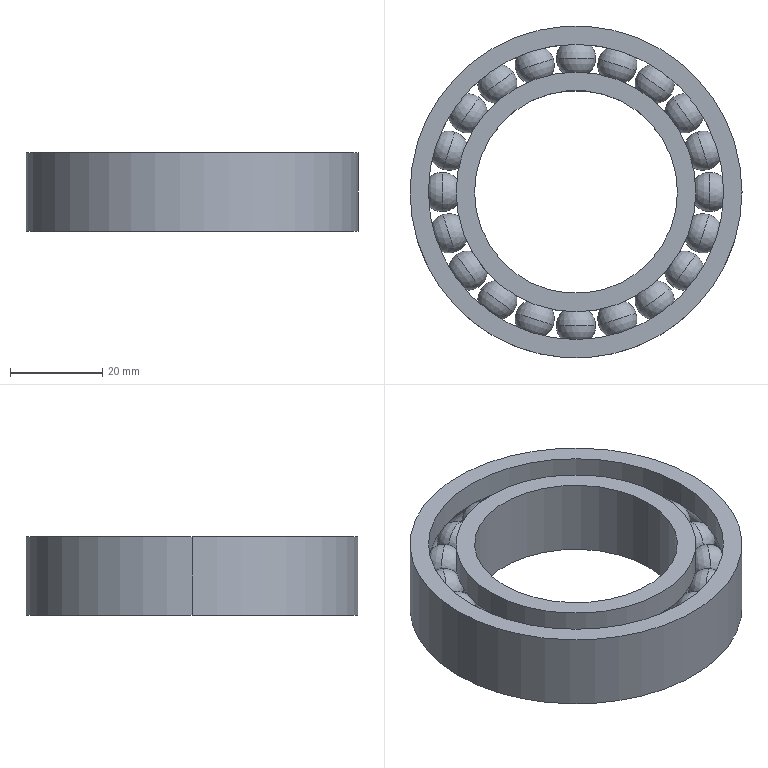Part | NX | features BREP 22 | 22 solids | 102 faces | box 72 x 72 x 17 mm | volume 29322 mm3 | sphere 80 | cylinder 12 | torus 6 | plane 4 | commonest cylinder face diameters 52 x4 64 x4 44 x2 72 x2